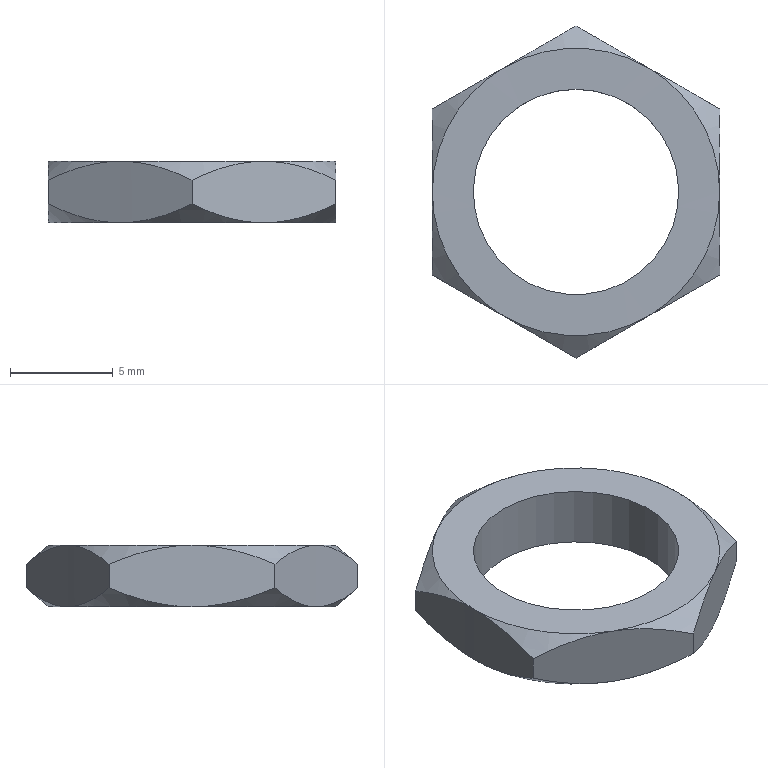Part | STEP file | 1-73.2 | 1 solid | 21 faces | box 14 x 16.166 x 3 mm | volume 263.877 mm3 | cone 12 | plane 8 | cylinder 1 | commonest cylinder face diameters 10 x1